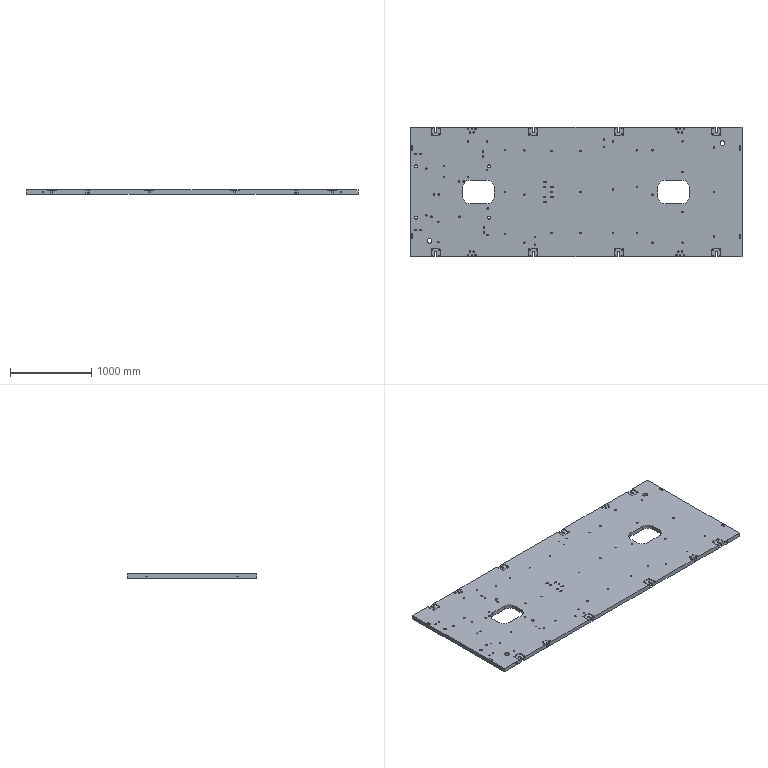Part | NX | features solid 2 | 1 solid | 416 faces | box 4080 x 1595 x 50 mm | volume 311286934 mm3 | cylinder 230 | plane 130 | cone 56 | commonest cylinder face diameters 18 x52 27 x52 8.5 x32 17.5 x20 24 x16 18.008 x12